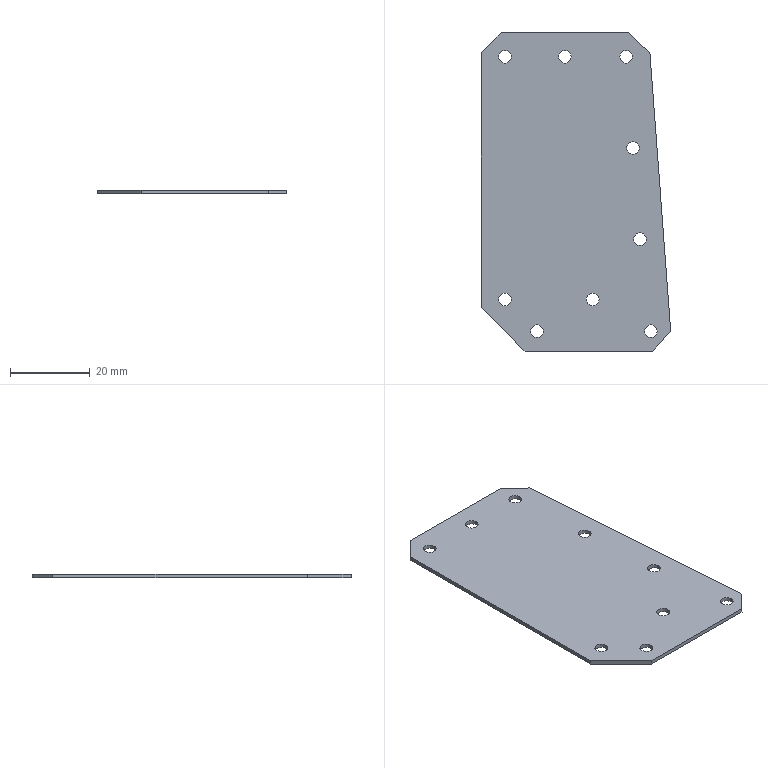Part | SolidWorks | features BaseBody 1 | 1 solid | 28 faces | box 47.626 x 80 x 1 mm | volume 3430 mm3 | cylinder 18 | plane 10 | commonest cylinder face diameters 3.2 x18
STEP:
#1=CARTESIAN_POINT('',(41.473,28.129,-1.));
#2=VERTEX_POINT('',#1);
#3=CARTESIAN_POINT('',(38.273,28.129,-1.));
#4=VERTEX_POINT('',#3);
#5=CARTESIAN_POINT('',(39.873,28.129,-1.));
#6=DIRECTION('',(0.,0.,-1.));
#7=DIRECTION('',(1.,0.,0.));
#8=AXIS2_PLACEMENT_3D('',#5,#6,#7);
#9=CIRCLE('',#8,1.6);
#10=EDGE_CURVE('',#2,#4,#9,.T.);
#11=ORIENTED_EDGE('',*,*,#10,.T.);
#12=CARTESIAN_POINT('',(38.273,28.129,0.));
#13=VERTEX_POINT('',#12);
#14=CARTESIAN_POINT('',(38.273,28.129,-1.));
#15=DIRECTION('',(0.,0.,1.));
#16=VECTOR('',#15,1000.);
#17=LINE('',#14,#16);
#18=EDGE_CURVE('',#4,#13,#17,.T.);
#19=ORIENTED_EDGE('',*,*,#18,.T.);
#20=CARTESIAN_POINT('',(41.473,28.129,0.));
#21=VERTEX_POINT('',#20);
#22=CARTESIAN_POINT('',(39.873,28.129,0.));
#23=DIRECTION('',(0.,0.,1.));
#24=DIRECTION('',(1.,0.,0.));
#25=AXIS2_PLACEMENT_3D('',#22,#23,#24);
#26=CIRCLE('',#25,1.6);
#27=EDGE_CURVE('',#13,#21,#26,.T.);
#28=ORIENTED_EDGE('',*,*,#27,.T.);
#29=CARTESIAN_POINT('',(41.473,28.129,-1.));
#30=DIRECTION('',(0.,0.,1.));
#31=VECTOR('',#30,1000.);
#32=LINE('',#29,#31);
#33=EDGE_CURVE('',#2,#21,#32,.T.);
#34=ORIENTED_EDGE('',*,*,#33,.F.);
#35=EDGE_LOOP('',(#11,#19,#28,#34));
#36=FACE_OUTER_BOUND('',#35,.T.);
#37=CARTESIAN_POINT('',(39.873,28.129,-1.));
#38=DIRECTION('',(0.,0.,1.));
#39=DIRECTION('',(1.,0.,0.));
#40=AXIS2_PLACEMENT_3D('',#37,#38,#39);
#41=CYLINDRICAL_SURFACE('',#40,1.6);
#42=ADVANCED_FACE('',(#36),#41,.F.);
#43=CARTESIAN_POINT('',(44.211,5.,-1.));
#44=VERTEX_POINT('',#43);
#45=CARTESIAN_POINT('',(41.011,5.,-1.));
#46=VERTEX_POINT('',#45);
#47=CARTESIAN_POINT('',(42.611,5.,-1.));
#48=DIRECTION('',(0.,0.,-1.));
#49=DIRECTION('',(1.,0.,0.));
#50=AXIS2_PLACEMENT_3D('',#47,#48,#49);
#51=CIRCLE('',#50,1.6);
#52=EDGE_CURVE('',#44,#46,#51,.T.);
#53=ORIENTED_EDGE('',*,*,#52,.T.);
#54=CARTESIAN_POINT('',(41.011,5.,0.));
#55=VERTEX_POINT('',#54);
#56=CARTESIAN_POINT('',(41.011,5.,-1.));
#57=DIRECTION('',(0.,0.,1.));
#58=VECTOR('',#57,1000.);
#59=LINE('',#56,#58);
#60=EDGE_CURVE('',#46,#55,#59,.T.);
#61=ORIENTED_EDGE('',*,*,#60,.T.);
#62=CARTESIAN_POINT('',(44.211,5.,0.));
#63=VERTEX_POINT('',#62);
#64=CARTESIAN_POINT('',(42.611,5.,0.));
#65=DIRECTION('',(0.,0.,-1.));
#66=DIRECTION('',(1.,0.,0.));
#67=AXIS2_PLACEMENT_3D('',#64,#65,#66);
#68=CIRCLE('',#67,1.6);
#69=EDGE_CURVE('',#63,#55,#68,.T.);
#70=ORIENTED_EDGE('',*,*,#69,.F.);
#71=CARTESIAN_POINT('',(44.211,5.,-1.));
#72=DIRECTION('',(0.,0.,1.));
#73=VECTOR('',#72,1000.);
#74=LINE('',#71,#73);
#75=EDGE_CURVE('',#44,#63,#74,.T.);
#76=ORIENTED_EDGE('',*,*,#75,.F.);
#77=EDGE_LOOP('',(#53,#61,#70,#76));
#78=FACE_OUTER_BOUND('',#77,.T.);
#79=CARTESIAN_POINT('',(42.611,5.,-1.));
#80=DIRECTION('',(0.,0.,1.));
#81=DIRECTION('',(1.,0.,0.));
#82=AXIS2_PLACEMENT_3D('',#79,#80,#81);
#83=CYLINDRICAL_SURFACE('',#82,1.6);
#84=ADVANCED_FACE('',(#78),#83,.F.);
#85=CARTESIAN_POINT('',(15.6,5.,-1.));
#86=VERTEX_POINT('',#85);
#87=CARTESIAN_POINT('',(12.4,5.,-1.));
#88=VERTEX_POINT('',#87);
#89=CARTESIAN_POINT('',(14.,5.,-1.));
#90=DIRECTION('',(0.,0.,-1.));
#91=DIRECTION('',(1.,0.,0.));
#92=AXIS2_PLACEMENT_3D('',#89,#90,#91);
#93=CIRCLE('',#92,1.6);
#94=EDGE_CURVE('',#86,#88,#93,.T.);
#95=ORIENTED_EDGE('',*,*,#94,.T.);
#96=CARTESIAN_POINT('',(12.4,5.,0.));
#97=VERTEX_POINT('',#96);
#98=CARTESIAN_POINT('',(12.4,5.,-1.));
#99=DIRECTION('',(0.,0.,1.));
#100=VECTOR('',#99,1000.);
#101=LINE('',#98,#100);
#102=EDGE_CURVE('',#88,#97,#101,.T.);
#103=ORIENTED_EDGE('',*,*,#102,.T.);
#104=CARTESIAN_POINT('',(15.6,5.,0.));
#105=VERTEX_POINT('',#104);
#106=CARTESIAN_POINT('',(14.,5.,0.));
#107=DIRECTION('',(0.,0.,-1.));
#108=DIRECTION('',(1.,0.,0.));
#109=AXIS2_PLACEMENT_3D('',#106,#107,#108);
#110=CIRCLE('',#109,1.6);
#111=EDGE_CURVE('',#105,#97,#110,.T.);
#112=ORIENTED_EDGE('',*,*,#111,.F.);
#113=CARTESIAN_POINT('',(15.6,5.,-1.));
#114=DIRECTION('',(0.,0.,1.));
#115=VECTOR('',#114,1000.);
#116=LINE('',#113,#115);
#117=EDGE_CURVE('',#86,#105,#116,.T.);
#118=ORIENTED_EDGE('',*,*,#117,.F.);
#119=EDGE_LOOP('',(#95,#103,#112,#118));
#120=FACE_OUTER_BOUND('',#119,.T.);
#121=CARTESIAN_POINT('',(14.,5.,-1.));
#122=DIRECTION('',(0.,0.,1.));
#123=DIRECTION('',(1.,0.,0.));
#124=AXIS2_PLACEMENT_3D('',#121,#122,#123);
#125=CYLINDRICAL_SURFACE('',#124,1.6);
#126=ADVANCED_FACE('',(#120),#125,.F.);
#127=CARTESIAN_POINT('',(7.6,13.,-1.));
#128=VERTEX_POINT('',#127);
#129=CARTESIAN_POINT('',(4.4,13.,-1.));
#130=VERTEX_POINT('',#129);
#131=CARTESIAN_POINT('',(6.,13.,-1.));
#132=DIRECTION('',(0.,0.,-1.));
#133=DIRECTION('',(1.,0.,0.));
#134=AXIS2_PLACEMENT_3D('',#131,#132,#133);
#135=CIRCLE('',#134,1.6);
#136=EDGE_CURVE('',#128,#130,#135,.T.);
#137=ORIENTED_EDGE('',*,*,#136,.T.);
#138=CARTESIAN_POINT('',(4.4,13.,0.));
#139=VERTEX_POINT('',#138);
#140=CARTESIAN_POINT('',(4.4,13.,-1.));
#141=DIRECTION('',(0.,0.,1.));
#142=VECTOR('',#141,1000.);
#143=LINE('',#140,#142);
#144=EDGE_CURVE('',#130,#139,#143,.T.);
#145=ORIENTED_EDGE('',*,*,#144,.T.);
#146=CARTESIAN_POINT('',(7.6,13.,0.));
#147=VERTEX_POINT('',#146);
#148=CARTESIAN_POINT('',(6.,13.,0.));
#149=DIRECTION('',(0.,0.,-1.));
#150=DIRECTION('',(1.,0.,0.));
#151=AXIS2_PLACEMENT_3D('',#148,#149,#150);
#152=CIRCLE('',#151,1.6);
#153=EDGE_CURVE('',#147,#139,#152,.T.);
#154=ORIENTED_EDGE('',*,*,#153,.F.);
#155=CARTESIAN_POINT('',(7.6,13.,-1.));
#156=DIRECTION('',(0.,0.,1.));
#157=VECTOR('',#156,1000.);
#158=LINE('',#155,#157);
#159=EDGE_CURVE('',#128,#147,#158,.T.);
#160=ORIENTED_EDGE('',*,*,#159,.F.);
#161=EDGE_LOOP('',(#137,#145,#154,#160));
#162=FACE_OUTER_BOUND('',#161,.T.);
#163=CARTESIAN_POINT('',(6.,13.,-1.));
#164=DIRECTION('',(0.,0.,1.));
#165=DIRECTION('',(1.,0.,0.));
#166=AXIS2_PLACEMENT_3D('',#163,#164,#165);
#167=CYLINDRICAL_SURFACE('',#166,1.6);
#168=ADVANCED_FACE('',(#162),#167,.F.);
#169=CARTESIAN_POINT('',(29.6,13.,-1.));
#170=VERTEX_POINT('',#169);
#171=CARTESIAN_POINT('',(26.4,13.,-1.));
#172=VERTEX_POINT('',#171);
#173=CARTESIAN_POINT('',(28.,13.,-1.));
#174=DIRECTION('',(0.,0.,-1.));
#175=DIRECTION('',(1.,0.,0.));
#176=AXIS2_PLACEMENT_3D('',#173,#174,#175);
#177=CIRCLE('',#176,1.6);
#178=EDGE_CURVE('',#170,#172,#177,.T.);
#179=ORIENTED_EDGE('',*,*,#178,.T.);
#180=CARTESIAN_POINT('',(26.4,13.,0.));
#181=VERTEX_POINT('',#180);
#182=CARTESIAN_POINT('',(26.4,13.,-1.));
#183=DIRECTION('',(0.,0.,1.));
#184=VECTOR('',#183,1000.);
#185=LINE('',#182,#184);
#186=EDGE_CURVE('',#172,#181,#185,.T.);
#187=ORIENTED_EDGE('',*,*,#186,.T.);
#188=CARTESIAN_POINT('',(29.6,13.,0.));
#189=VERTEX_POINT('',#188);
#190=CARTESIAN_POINT('',(28.,13.,0.));
#191=DIRECTION('',(0.,0.,-1.));
#192=DIRECTION('',(1.,0.,0.));
#193=AXIS2_PLACEMENT_3D('',#190,#191,#192);
#194=CIRCLE('',#193,1.6);
#195=EDGE_CURVE('',#189,#181,#194,.T.);
#196=ORIENTED_EDGE('',*,*,#195,.F.);
#197=CARTESIAN_POINT('',(29.6,13.,-1.));
#198=DIRECTION('',(0.,0.,1.));
#199=VECTOR('',#198,1000.);
#200=LINE('',#197,#199);
#201=EDGE_CURVE('',#170,#189,#200,.T.);
#202=ORIENTED_EDGE('',*,*,#201,.F.);
#203=EDGE_LOOP('',(#179,#187,#196,#202));
#204=FACE_OUTER_BOUND('',#203,.T.);
#205=CARTESIAN_POINT('',(28.,13.,-1.));
#206=DIRECTION('',(0.,0.,1.));
#207=DIRECTION('',(1.,0.,0.));
#208=AXIS2_PLACEMENT_3D('',#205,#206,#207);
#209=CYLINDRICAL_SURFACE('',#208,1.6);
#210=ADVANCED_FACE('',(#204),#209,.F.);
#211=CARTESIAN_POINT('',(7.6,74.,-1.));
#212=VERTEX_POINT('',#211);
#213=CARTESIAN_POINT('',(4.4,74.,-1.));
#214=VERTEX_POINT('',#213);
#215=CARTESIAN_POINT('',(6.,74.,-1.));
#216=DIRECTION('',(0.,0.,-1.));
#217=DIRECTION('',(1.,0.,0.));
#218=AXIS2_PLACEMENT_3D('',#215,#216,#217);
#219=CIRCLE('',#218,1.6);
#220=EDGE_CURVE('',#212,#214,#219,.T.);
#221=ORIENTED_EDGE('',*,*,#220,.T.);
#222=CARTESIAN_POINT('',(4.4,74.,0.));
#223=VERTEX_POINT('',#222);
#224=CARTESIAN_POINT('',(4.4,74.,-1.));
#225=DIRECTION('',(0.,0.,1.));
#226=VECTOR('',#225,1000.);
#227=LINE('',#224,#226);
#228=EDGE_CURVE('',#214,#223,#227,.T.);
#229=ORIENTED_EDGE('',*,*,#228,.T.);
#230=CARTESIAN_POINT('',(7.6,74.,0.));
#231=VERTEX_POINT('',#230);
#232=CARTESIAN_POINT('',(6.,74.,0.));
#233=DIRECTION('',(0.,0.,-1.));
#234=DIRECTION('',(1.,0.,0.));
#235=AXIS2_PLACEMENT_3D('',#232,#233,#234);
#236=CIRCLE('',#235,1.6);
#237=EDGE_CURVE('',#231,#223,#236,.T.);
#238=ORIENTED_EDGE('',*,*,#237,.F.);
#239=CARTESIAN_POINT('',(7.6,74.,-1.));
#240=DIRECTION('',(0.,0.,1.));
#241=VECTOR('',#240,1000.);
#242=LINE('',#239,#241);
#243=EDGE_CURVE('',#212,#231,#242,.T.);
#244=ORIENTED_EDGE('',*,*,#243,.F.);
#245=EDGE_LOOP('',(#221,#229,#238,#244));
#246=FACE_OUTER_BOUND('',#245,.T.);
#247=CARTESIAN_POINT('',(6.,74.,-1.));
#248=DIRECTION('',(0.,0.,1.));
#249=DIRECTION('',(1.,0.,0.));
#250=AXIS2_PLACEMENT_3D('',#247,#248,#249);
#251=CYLINDRICAL_SURFACE('',#250,1.6);
#252=ADVANCED_FACE('',(#246),#251,.F.);
#253=CARTESIAN_POINT('',(22.6,74.,-1.));
#254=VERTEX_POINT('',#253);
#255=CARTESIAN_POINT('',(19.4,74.,-1.));
#256=VERTEX_POINT('',#255);
#257=CARTESIAN_POINT('',(21.,74.,-1.));
#258=DIRECTION('',(0.,0.,-1.));
#259=DIRECTION('',(1.,0.,0.));
#260=AXIS2_PLACEMENT_3D('',#257,#258,#259);
#261=CIRCLE('',#260,1.6);
#262=EDGE_CURVE('',#254,#256,#261,.T.);
#263=ORIENTED_EDGE('',*,*,#262,.T.);
#264=CARTESIAN_POINT('',(19.4,74.,0.));
#265=VERTEX_POINT('',#264);
#266=CARTESIAN_POINT('',(19.4,74.,-1.));
#267=DIRECTION('',(0.,0.,1.));
#268=VECTOR('',#267,1000.);
#269=LINE('',#266,#268);
#270=EDGE_CURVE('',#256,#265,#269,.T.);
#271=ORIENTED_EDGE('',*,*,#270,.T.);
#272=CARTESIAN_POINT('',(22.6,74.,0.));
#273=VERTEX_POINT('',#272);
#274=CARTESIAN_POINT('',(21.,74.,0.));
#275=DIRECTION('',(0.,0.,-1.));
#276=DIRECTION('',(1.,0.,0.));
#277=AXIS2_PLACEMENT_3D('',#274,#275,#276);
#278=CIRCLE('',#277,1.6);
#279=EDGE_CURVE('',#273,#265,#278,.T.);
#280=ORIENTED_EDGE('',*,*,#279,.F.);
#281=CARTESIAN_POINT('',(22.6,74.,-1.));
#282=DIRECTION('',(0.,0.,1.));
#283=VECTOR('',#282,1000.);
#284=LINE('',#281,#283);
#285=EDGE_CURVE('',#254,#273,#284,.T.);
#286=ORIENTED_EDGE('',*,*,#285,.F.);
#287=EDGE_LOOP('',(#263,#271,#280,#286));
#288=FACE_OUTER_BOUND('',#287,.T.);
#289=CARTESIAN_POINT('',(21.,74.,-1.));
#290=DIRECTION('',(0.,0.,1.));
#291=DIRECTION('',(1.,0.,0.));
#292=AXIS2_PLACEMENT_3D('',#289,#290,#291);
#293=CYLINDRICAL_SURFACE('',#292,1.6);
#294=ADVANCED_FACE('',(#288),#293,.F.);
#295=CARTESIAN_POINT('',(38.033,74.,-1.));
#296=VERTEX_POINT('',#295);
#297=CARTESIAN_POINT('',(34.833,74.,-1.));
#298=VERTEX_POINT('',#297);
#299=CARTESIAN_POINT('',(36.433,74.,-1.));
#300=DIRECTION('',(0.,0.,-1.));
#301=DIRECTION('',(1.,0.,0.));
#302=AXIS2_PLACEMENT_3D('',#299,#300,#301);
#303=CIRCLE('',#302,1.6);
#304=EDGE_CURVE('',#296,#298,#303,.T.);
#305=ORIENTED_EDGE('',*,*,#304,.T.);
#306=CARTESIAN_POINT('',(34.833,74.,0.));
#307=VERTEX_POINT('',#306);
#308=CARTESIAN_POINT('',(34.833,74.,-1.));
#309=DIRECTION('',(0.,0.,1.));
#310=VECTOR('',#309,1000.);
#311=LINE('',#308,#310);
#312=EDGE_CURVE('',#298,#307,#311,.T.);
#313=ORIENTED_EDGE('',*,*,#312,.T.);
#314=CARTESIAN_POINT('',(38.033,74.,0.));
#315=VERTEX_POINT('',#314);
#316=CARTESIAN_POINT('',(36.433,74.,0.));
#317=DIRECTION('',(0.,0.,-1.));
#318=DIRECTION('',(1.,0.,0.));
#319=AXIS2_PLACEMENT_3D('',#316,#317,#318);
#320=CIRCLE('',#319,1.6);
#321=EDGE_CURVE('',#315,#307,#320,.T.);
#322=ORIENTED_EDGE('',*,*,#321,.F.);
#323=CARTESIAN_POINT('',(38.033,74.,-1.));
#324=DIRECTION('',(0.,0.,1.));
#325=VECTOR('',#324,1000.);
#326=LINE('',#323,#325);
#327=EDGE_CURVE('',#296,#315,#326,.T.);
#328=ORIENTED_EDGE('',*,*,#327,.F.);
#329=EDGE_LOOP('',(#305,#313,#322,#328));
#330=FACE_OUTER_BOUND('',#329,.T.);
#331=CARTESIAN_POINT('',(36.433,74.,-1.));
#332=DIRECTION('',(0.,0.,1.));
#333=DIRECTION('',(1.,0.,0.));
#334=AXIS2_PLACEMENT_3D('',#331,#332,#333);
#335=CYLINDRICAL_SURFACE('',#334,1.6);
#336=ADVANCED_FACE('',(#330),#335,.F.);
#337=CARTESIAN_POINT('',(39.753,51.064,-1.));
#338=VERTEX_POINT('',#337);
#339=CARTESIAN_POINT('',(36.553,51.064,-1.));
#340=VERTEX_POINT('',#339);
#341=CARTESIAN_POINT('',(38.153,51.064,-1.));
#342=DIRECTION('',(0.,0.,-1.));
#343=DIRECTION('',(1.,0.,0.));
#344=AXIS2_PLACEMENT_3D('',#341,#342,#343);
#345=CIRCLE('',#344,1.6);
#346=EDGE_CURVE('',#338,#340,#345,.T.);
#347=ORIENTED_EDGE('',*,*,#346,.T.);
#348=CARTESIAN_POINT('',(36.553,51.064,0.));
#349=VERTEX_POINT('',#348);
#350=CARTESIAN_POINT('',(36.553,51.064,-1.));
#351=DIRECTION('',(0.,0.,1.));
#352=VECTOR('',#351,1000.);
#353=LINE('',#350,#352);
#354=EDGE_CURVE('',#340,#349,#353,.T.);
#355=ORIENTED_EDGE('',*,*,#354,.T.);
#356=CARTESIAN_POINT('',(39.753,51.064,0.));
#357=VERTEX_POINT('',#356);
#358=CARTESIAN_POINT('',(38.153,51.064,0.));
#359=DIRECTION('',(0.,0.,-1.));
#360=DIRECTION('',(1.,0.,0.));
#361=AXIS2_PLACEMENT_3D('',#358,#359,#360);
#362=CIRCLE('',#361,1.6);
#363=EDGE_CURVE('',#357,#349,#362,.T.);
#364=ORIENTED_EDGE('',*,*,#363,.F.);
#365=CARTESIAN_POINT('',(39.753,51.064,-1.));
#366=DIRECTION('',(0.,0.,1.));
#367=VECTOR('',#366,1000.);
#368=LINE('',#365,#367);
#369=EDGE_CURVE('',#338,#357,#368,.T.);
#370=ORIENTED_EDGE('',*,*,#369,.F.);
#371=EDGE_LOOP('',(#347,#355,#364,#370));
#372=FACE_OUTER_BOUND('',#371,.T.);
#373=CARTESIAN_POINT('',(38.153,51.064,-1.));
#374=DIRECTION('',(0.,0.,1.));
#375=DIRECTION('',(1.,0.,0.));
#376=AXIS2_PLACEMENT_3D('',#373,#374,#375);
#377=CYLINDRICAL_SURFACE('',#376,1.6);
#378=ADVANCED_FACE('',(#372),#377,.F.);
#379=ORIENTED_EDGE('',*,*,#18,.F.);
#380=CARTESIAN_POINT('',(39.873,28.129,-1.));
#381=DIRECTION('',(0.,0.,-1.));
#382=DIRECTION('',(1.,0.,0.));
#383=AXIS2_PLACEMENT_3D('',#380,#381,#382);
#384=CIRCLE('',#383,1.6);
#385=EDGE_CURVE('',#4,#2,#384,.T.);
#386=ORIENTED_EDGE('',*,*,#385,.T.);
#387=ORIENTED_EDGE('',*,*,#33,.T.);
#388=CARTESIAN_POINT('',(39.873,28.129,0.));
#389=DIRECTION('',(0.,0.,1.));
#390=DIRECTION('',(1.,0.,0.));
#391=AXIS2_PLACEMENT_3D('',#388,#389,#390);
#392=CIRCLE('',#391,1.6);
#393=EDGE_CURVE('',#21,#13,#392,.T.);
#394=ORIENTED_EDGE('',*,*,#393,.T.);
#395=EDGE_LOOP('',(#379,#386,#387,#394));
#396=FACE_OUTER_BOUND('',#395,.T.);
#397=CARTESIAN_POINT('',(39.873,28.129,-1.));
#398=DIRECTION('',(0.,0.,1.));
#399=DIRECTION('',(1.,0.,0.));
#400=AXIS2_PLACEMENT_3D('',#397,#398,#399);
#401=CYLINDRICAL_SURFACE('',#400,1.6);
#402=ADVANCED_FACE('',(#396),#401,.F.);
#403=ORIENTED_EDGE('',*,*,#69,.T.);
#404=CARTESIAN_POINT('',(42.611,5.,0.));
#405=DIRECTION('',(0.,0.,-1.));
#406=DIRECTION('',(1.,0.,0.));
#407=AXIS2_PLACEMENT_3D('',#404,#405,#406);
#408=CIRCLE('',#407,1.6);
#409=EDGE_CURVE('',#55,#63,#408,.T.);
#410=ORIENTED_EDGE('',*,*,#409,.T.);
#411=EDGE_LOOP('',(#403,#410));
#412=FACE_BOUND('',#411,.T.);
#413=ORIENTED_EDGE('',*,*,#111,.T.);
#414=CARTESIAN_POINT('',(14.,5.,0.));
#415=DIRECTION('',(0.,0.,-1.));
#416=DIRECTION('',(1.,0.,0.));
#417=AXIS2_PLACEMENT_3D('',#414,#415,#416);
#418=CIRCLE('',#417,1.6);
#419=EDGE_CURVE('',#97,#105,#418,.T.);
#420=ORIENTED_EDGE('',*,*,#419,.T.);
#421=EDGE_LOOP('',(#413,#420));
#422=FACE_BOUND('',#421,.T.);
#423=ORIENTED_EDGE('',*,*,#153,.T.);
#424=CARTESIAN_POINT('',(6.,13.,0.));
#425=DIRECTION('',(0.,0.,-1.));
#426=DIRECTION('',(1.,0.,0.));
#427=AXIS2_PLACEMENT_3D('',#424,#425,#426);
#428=CIRCLE('',#427,1.6);
#429=EDGE_CURVE('',#139,#147,#428,.T.);
#430=ORIENTED_EDGE('',*,*,#429,.T.);
#431=EDGE_LOOP('',(#423,#430));
#432=FACE_BOUND('',#431,.T.);
#433=ORIENTED_EDGE('',*,*,#195,.T.);
#434=CARTESIAN_POINT('',(28.,13.,0.));
#435=DIRECTION('',(0.,0.,-1.));
#436=DIRECTION('',(1.,0.,0.));
#437=AXIS2_PLACEMENT_3D('',#434,#435,#436);
#438=CIRCLE('',#437,1.6);
#439=EDGE_CURVE('',#181,#189,#438,.T.);
#440=ORIENTED_EDGE('',*,*,#439,.T.);
#441=EDGE_LOOP('',(#433,#440));
#442=FACE_BOUND('',#441,.T.);
#443=ORIENTED_EDGE('',*,*,#237,.T.);
#444=CARTESIAN_POINT('',(6.,74.,0.));
#445=DIRECTION('',(0.,0.,-1.));
#446=DIRECTION('',(1.,0.,0.));
#447=AXIS2_PLACEMENT_3D('',#444,#445,#446);
#448=CIRCLE('',#447,1.6);
#449=EDGE_CURVE('',#223,#231,#448,.T.);
#450=ORIENTED_EDGE('',*,*,#449,.T.);
#451=EDGE_LOOP('',(#443,#450));
#452=FACE_BOUND('',#451,.T.);
#453=ORIENTED_EDGE('',*,*,#279,.T.);
#454=CARTESIAN_POINT('',(21.,74.,0.));
#455=DIRECTION('',(0.,0.,-1.));
#456=DIRECTION('',(1.,0.,0.));
#457=AXIS2_PLACEMENT_3D('',#454,#455,#456);
#458=CIRCLE('',#457,1.6);
#459=EDGE_CURVE('',#265,#273,#458,.T.);
#460=ORIENTED_EDGE('',*,*,#459,.T.);
#461=EDGE_LOOP('',(#453,#460));
#462=FACE_BOUND('',#461,.T.);
#463=ORIENTED_EDGE('',*,*,#321,.T.);
#464=CARTESIAN_POINT('',(36.433,74.,0.));
#465=DIRECTION('',(0.,0.,-1.));
#466=DIRECTION('',(1.,0.,0.));
#467=AXIS2_PLACEMENT_3D('',#464,#465,#466);
#468=CIRCLE('',#467,1.6);
#469=EDGE_CURVE('',#307,#315,#468,.T.);
#470=ORIENTED_EDGE('',*,*,#469,.T.);
#471=EDGE_LOOP('',(#463,#470));
#472=FACE_BOUND('',#471,.T.);
#473=ORIENTED_EDGE('',*,*,#363,.T.);
#474=CARTESIAN_POINT('',(38.153,51.064,0.));
#475=DIRECTION('',(0.,0.,-1.));
#476=DIRECTION('',(1.,0.,0.));
#477=AXIS2_PLACEMENT_3D('',#474,#475,#476);
#478=CIRCLE('',#477,1.6);
#479=EDGE_CURVE('',#349,#357,#478,.T.);
#480=ORIENTED_EDGE('',*,*,#479,.T.);
#481=EDGE_LOOP('',(#473,#480));
#482=FACE_BOUND('',#481,.T.);
#483=ORIENTED_EDGE('',*,*,#393,.F.);
#484=ORIENTED_EDGE('',*,*,#27,.F.);
#485=EDGE_LOOP('',(#483,#484));
#486=FACE_BOUND('',#485,.T.);
#487=CARTESIAN_POINT('',(0.,75.,0.));
#488=VERTEX_POINT('',#487);
#489=CARTESIAN_POINT('',(0.,11.,0.));
#490=VERTEX_POINT('',#489);
#491=CARTESIAN_POINT('',(0.,40.,0.));
#492=DIRECTION('',(0.,-1.,0.));
#493=VECTOR('',#492,1000.);
#494=LINE('',#491,#493);
#495=EDGE_CURVE('',#488,#490,#494,.T.);
#496=ORIENTED_EDGE('',*,*,#495,.T.);
#497=CARTESIAN_POINT('',(11.,0.,0.));
#498=VERTEX_POINT('',#497);
#499=CARTESIAN_POINT('',(0.,11.,0.));
#500=DIRECTION('',(0.7071,-0.7071,0.));
#501=VECTOR('',#500,1000.);
#502=LINE('',#499,#501);
#503=EDGE_CURVE('',#490,#498,#502,.T.);
#504=ORIENTED_EDGE('',*,*,#503,.T.);
#505=CARTESIAN_POINT('',(43.,0.,0.));
#506=VERTEX_POINT('',#505);
#507=CARTESIAN_POINT('',(23.956,0.,0.));
#508=DIRECTION('',(1.,0.,0.));
#509=VECTOR('',#508,1000.);
#510=LINE('',#507,#509);
#511=EDGE_CURVE('',#498,#506,#510,.T.);
#512=ORIENTED_EDGE('',*,*,#511,.T.);
#513=CARTESIAN_POINT('',(47.626,4.986,0.));
#514=VERTEX_POINT('',#513);
#515=CARTESIAN_POINT('',(43.,0.,0.));
#516=DIRECTION('',(0.6802,0.7331,0.));
#517=VECTOR('',#516,1000.);
#518=LINE('',#515,#517);
#519=EDGE_CURVE('',#506,#514,#518,.T.);
#520=ORIENTED_EDGE('',*,*,#519,.T.);
#521=CARTESIAN_POINT('',(42.374,75.014,0.));
#522=VERTEX_POINT('',#521);
#523=CARTESIAN_POINT('',(47.626,4.986,0.));
#524=DIRECTION('',(-0.07479,0.9972,0.));
#525=VECTOR('',#524,1000.);
#526=LINE('',#523,#525);
#527=EDGE_CURVE('',#514,#522,#526,.T.);
#528=ORIENTED_EDGE('',*,*,#527,.T.);
#529=CARTESIAN_POINT('',(37.,80.,0.));
#530=VERTEX_POINT('',#529);
#531=CARTESIAN_POINT('',(42.374,75.014,0.));
#532=DIRECTION('',(-0.7331,0.6802,0.));
#533=VECTOR('',#532,1000.);
#534=LINE('',#531,#533);
#535=EDGE_CURVE('',#522,#530,#534,.T.);
#536=ORIENTED_EDGE('',*,*,#535,.T.);
#537=CARTESIAN_POINT('',(5.,80.,0.));
#538=VERTEX_POINT('',#537);
#539=CARTESIAN_POINT('',(23.956,80.,0.));
#540=DIRECTION('',(-1.,0.,0.));
#541=VECTOR('',#540,1000.);
#542=LINE('',#539,#541);
#543=EDGE_CURVE('',#530,#538,#542,.T.);
#544=ORIENTED_EDGE('',*,*,#543,.T.);
#545=CARTESIAN_POINT('',(5.,80.,0.));
#546=DIRECTION('',(-0.7071,-0.7071,0.));
#547=VECTOR('',#546,1000.);
#548=LINE('',#545,#547);
#549=EDGE_CURVE('',#538,#488,#548,.T.);
#550=ORIENTED_EDGE('',*,*,#549,.T.);
#551=EDGE_LOOP('',(#496,#504,#512,#520,#528,#536,#544,#550));
#552=FACE_OUTER_BOUND('',#551,.T.);
#553=CARTESIAN_POINT('',(0.,0.,0.));
#554=DIRECTION('',(0.,0.,1.));
#555=DIRECTION('',(1.,0.,0.));
#556=AXIS2_PLACEMENT_3D('',#553,#554,#555);
#557=PLANE('',#556);
#558=ADVANCED_FACE('',(#412,#422,#432,#442,#452,#462,#472,#482,#486,#552),#557,.T.);
#559=ORIENTED_EDGE('',*,*,#52,.F.);
#560=CARTESIAN_POINT('',(42.611,5.,-1.));
#561=DIRECTION('',(0.,0.,-1.));
#562=DIRECTION('',(1.,0.,0.));
#563=AXIS2_PLACEMENT_3D('',#560,#561,#562);
#564=CIRCLE('',#563,1.6);
#565=EDGE_CURVE('',#46,#44,#564,.T.);
#566=ORIENTED_EDGE('',*,*,#565,.F.);
#567=EDGE_LOOP('',(#559,#566));
#568=FACE_BOUND('',#567,.T.);
#569=ORIENTED_EDGE('',*,*,#94,.F.);
#570=CARTESIAN_POINT('',(14.,5.,-1.));
#571=DIRECTION('',(0.,0.,-1.));
#572=DIRECTION('',(1.,0.,0.));
#573=AXIS2_PLACEMENT_3D('',#570,#571,#572);
#574=CIRCLE('',#573,1.6);
#575=EDGE_CURVE('',#88,#86,#574,.T.);
#576=ORIENTED_EDGE('',*,*,#575,.F.);
#577=EDGE_LOOP('',(#569,#576));
#578=FACE_BOUND('',#577,.T.);
#579=ORIENTED_EDGE('',*,*,#136,.F.);
#580=CARTESIAN_POINT('',(6.,13.,-1.));
#581=DIRECTION('',(0.,0.,-1.));
#582=DIRECTION('',(1.,0.,0.));
#583=AXIS2_PLACEMENT_3D('',#580,#581,#582);
#584=CIRCLE('',#583,1.6);
#585=EDGE_CURVE('',#130,#128,#584,.T.);
#586=ORIENTED_EDGE('',*,*,#585,.F.);
#587=EDGE_LOOP('',(#579,#586));
#588=FACE_BOUND('',#587,.T.);
#589=ORIENTED_EDGE('',*,*,#178,.F.);
#590=CARTESIAN_POINT('',(28.,13.,-1.));
#591=DIRECTION('',(0.,0.,-1.));
#592=DIRECTION('',(1.,0.,0.));
#593=AXIS2_PLACEMENT_3D('',#590,#591,#592);
#594=CIRCLE('',#593,1.6);
#595=EDGE_CURVE('',#172,#170,#594,.T.);
#596=ORIENTED_EDGE('',*,*,#595,.F.);
#597=EDGE_LOOP('',(#589,#596));
#598=FACE_BOUND('',#597,.T.);
#599=ORIENTED_EDGE('',*,*,#220,.F.);
#600=CARTESIAN_POINT('',(6.,74.,-1.));
#601=DIRECTION('',(0.,0.,-1.));
#602=DIRECTION('',(1.,0.,0.));
#603=AXIS2_PLACEMENT_3D('',#600,#601,#602);
#604=CIRCLE('',#603,1.6);
#605=EDGE_CURVE('',#214,#212,#604,.T.);
#606=ORIENTED_EDGE('',*,*,#605,.F.);
#607=EDGE_LOOP('',(#599,#606));
#608=FACE_BOUND('',#607,.T.);
#609=ORIENTED_EDGE('',*,*,#262,.F.);
#610=CARTESIAN_POINT('',(21.,74.,-1.));
#611=DIRECTION('',(0.,0.,-1.));
#612=DIRECTION('',(1.,0.,0.));
#613=AXIS2_PLACEMENT_3D('',#610,#611,#612);
#614=CIRCLE('',#613,1.6);
#615=EDGE_CURVE('',#256,#254,#614,.T.);
#616=ORIENTED_EDGE('',*,*,#615,.F.);
#617=EDGE_LOOP('',(#609,#616));
#618=FACE_BOUND('',#617,.T.);
#619=ORIENTED_EDGE('',*,*,#304,.F.);
#620=CARTESIAN_POINT('',(36.433,74.,-1.));
#621=DIRECTION('',(0.,0.,-1.));
#622=DIRECTION('',(1.,0.,0.));
#623=AXIS2_PLACEMENT_3D('',#620,#621,#622);
#624=CIRCLE('',#623,1.6);
#625=EDGE_CURVE('',#298,#296,#624,.T.);
#626=ORIENTED_EDGE('',*,*,#625,.F.);
#627=EDGE_LOOP('',(#619,#626));
#628=FACE_BOUND('',#627,.T.);
#629=ORIENTED_EDGE('',*,*,#346,.F.);
#630=CARTESIAN_POINT('',(38.153,51.064,-1.));
#631=DIRECTION('',(0.,0.,-1.));
#632=DIRECTION('',(1.,0.,0.));
#633=AXIS2_PLACEMENT_3D('',#630,#631,#632);
#634=CIRCLE('',#633,1.6);
#635=EDGE_CURVE('',#340,#338,#634,.T.);
#636=ORIENTED_EDGE('',*,*,#635,.F.);
#637=EDGE_LOOP('',(#629,#636));
#638=FACE_BOUND('',#637,.T.);
#639=ORIENTED_EDGE('',*,*,#10,.F.);
#640=ORIENTED_EDGE('',*,*,#385,.F.);
#641=EDGE_LOOP('',(#639,#640));
#642=FACE_BOUND('',#641,.T.);
#643=CARTESIAN_POINT('',(43.,0.,-1.));
#644=VERTEX_POINT('',#643);
#645=CARTESIAN_POINT('',(47.626,4.986,-1.));
#646=VERTEX_POINT('',#645);
#647=CARTESIAN_POINT('',(47.626,4.986,-1.));
#648=DIRECTION('',(0.6802,0.7331,0.));
#649=VECTOR('',#648,1000.);
#650=LINE('',#647,#649);
#651=EDGE_CURVE('',#644,#646,#650,.T.);
#652=ORIENTED_EDGE('',*,*,#651,.F.);
#653=CARTESIAN_POINT('',(11.,0.,-1.));
#654=VERTEX_POINT('',#653);
#655=CARTESIAN_POINT('',(23.956,0.,-1.));
#656=DIRECTION('',(1.,0.,0.));
#657=VECTOR('',#656,1000.);
#658=LINE('',#655,#657);
#659=EDGE_CURVE('',#654,#644,#658,.T.);
#660=ORIENTED_EDGE('',*,*,#659,.F.);
#661=CARTESIAN_POINT('',(0.,11.,-1.));
#662=VERTEX_POINT('',#661);
#663=CARTESIAN_POINT('',(0.,11.,-1.));
#664=DIRECTION('',(0.7071,-0.7071,0.));
#665=VECTOR('',#664,1000.);
#666=LINE('',#663,#665);
#667=EDGE_CURVE('',#662,#654,#666,.T.);
#668=ORIENTED_EDGE('',*,*,#667,.F.);
#669=CARTESIAN_POINT('',(0.,75.,-1.));
#670=VERTEX_POINT('',#669);
#671=CARTESIAN_POINT('',(0.,40.,-1.));
#672=DIRECTION('',(0.,-1.,0.));
#673=VECTOR('',#672,1000.);
#674=LINE('',#671,#673);
#675=EDGE_CURVE('',#670,#662,#674,.T.);
#676=ORIENTED_EDGE('',*,*,#675,.F.);
#677=CARTESIAN_POINT('',(5.,80.,-1.));
#678=VERTEX_POINT('',#677);
#679=CARTESIAN_POINT('',(0.,75.,-1.));
#680=DIRECTION('',(-0.7071,-0.7071,0.));
#681=VECTOR('',#680,1000.);
#682=LINE('',#679,#681);
#683=EDGE_CURVE('',#678,#670,#682,.T.);
#684=ORIENTED_EDGE('',*,*,#683,.F.);
#685=CARTESIAN_POINT('',(37.,80.,-1.));
#686=VERTEX_POINT('',#685);
#687=CARTESIAN_POINT('',(23.956,80.,-1.));
#688=DIRECTION('',(-1.,0.,0.));
#689=VECTOR('',#688,1000.);
#690=LINE('',#687,#689);
#691=EDGE_CURVE('',#686,#678,#690,.T.);
#692=ORIENTED_EDGE('',*,*,#691,.F.);
#693=CARTESIAN_POINT('',(42.374,75.014,-1.));
#694=VERTEX_POINT('',#693);
#695=CARTESIAN_POINT('',(37.,80.,-1.));
#696=DIRECTION('',(-0.7331,0.6802,0.));
#697=VECTOR('',#696,1000.);
#698=LINE('',#695,#697);
#699=EDGE_CURVE('',#694,#686,#698,.T.);
#700=ORIENTED_EDGE('',*,*,#699,.F.);
#701=CARTESIAN_POINT('',(47.626,4.986,-1.));
#702=DIRECTION('',(-0.07479,0.9972,0.));
#703=VECTOR('',#702,1000.);
#704=LINE('',#701,#703);
#705=EDGE_CURVE('',#646,#694,#704,.T.);
#706=ORIENTED_EDGE('',*,*,#705,.F.);
#707=EDGE_LOOP('',(#652,#660,#668,#676,#684,#692,#700,#706));
#708=FACE_OUTER_BOUND('',#707,.T.);
#709=CARTESIAN_POINT('',(0.,0.,-1.));
#710=DIRECTION('',(0.,0.,1.));
#711=DIRECTION('',(1.,0.,0.));
#712=AXIS2_PLACEMENT_3D('',#709,#710,#711);
#713=PLANE('',#712);
#714=ADVANCED_FACE('',(#568,#578,#588,#598,#608,#618,#628,#638,#642,#708),#713,.F.);
#715=ORIENTED_EDGE('',*,*,#60,.F.);
#716=ORIENTED_EDGE('',*,*,#565,.T.);
#717=ORIENTED_EDGE('',*,*,#75,.T.);
#718=ORIENTED_EDGE('',*,*,#409,.F.);
#719=EDGE_LOOP('',(#715,#716,#717,#718));
#720=FACE_OUTER_BOUND('',#719,.T.);
#721=CARTESIAN_POINT('',(42.611,5.,-1.));
#722=DIRECTION('',(0.,0.,1.));
#723=DIRECTION('',(1.,0.,0.));
#724=AXIS2_PLACEMENT_3D('',#721,#722,#723);
#725=CYLINDRICAL_SURFACE('',#724,1.6);
#726=ADVANCED_FACE('',(#720),#725,.F.);
#727=ORIENTED_EDGE('',*,*,#102,.F.);
#728=ORIENTED_EDGE('',*,*,#575,.T.);
#729=ORIENTED_EDGE('',*,*,#117,.T.);
#730=ORIENTED_EDGE('',*,*,#419,.F.);
#731=EDGE_LOOP('',(#727,#728,#729,#730));
#732=FACE_OUTER_BOUND('',#731,.T.);
#733=CARTESIAN_POINT('',(14.,5.,-1.));
#734=DIRECTION('',(0.,0.,1.));
#735=DIRECTION('',(1.,0.,0.));
#736=AXIS2_PLACEMENT_3D('',#733,#734,#735);
#737=CYLINDRICAL_SURFACE('',#736,1.6);
#738=ADVANCED_FACE('',(#732),#737,.F.);
#739=ORIENTED_EDGE('',*,*,#144,.F.);
#740=ORIENTED_EDGE('',*,*,#585,.T.);
#741=ORIENTED_EDGE('',*,*,#159,.T.);
#742=ORIENTED_EDGE('',*,*,#429,.F.);
#743=EDGE_LOOP('',(#739,#740,#741,#742));
#744=FACE_OUTER_BOUND('',#743,.T.);
#745=CARTESIAN_POINT('',(6.,13.,-1.));
#746=DIRECTION('',(0.,0.,1.));
#747=DIRECTION('',(1.,0.,0.));
#748=AXIS2_PLACEMENT_3D('',#745,#746,#747);
#749=CYLINDRICAL_SURFACE('',#748,1.6);
#750=ADVANCED_FACE('',(#744),#749,.F.);
#751=ORIENTED_EDGE('',*,*,#186,.F.);
#752=ORIENTED_EDGE('',*,*,#595,.T.);
#753=ORIENTED_EDGE('',*,*,#201,.T.);
#754=ORIENTED_EDGE('',*,*,#439,.F.);
#755=EDGE_LOOP('',(#751,#752,#753,#754));
#756=FACE_OUTER_BOUND('',#755,.T.);
#757=CARTESIAN_POINT('',(28.,13.,-1.));
#758=DIRECTION('',(0.,0.,1.));
#759=DIRECTION('',(1.,0.,0.));
#760=AXIS2_PLACEMENT_3D('',#757,#758,#759);
#761=CYLINDRICAL_SURFACE('',#760,1.6);
#762=ADVANCED_FACE('',(#756),#761,.F.);
#763=ORIENTED_EDGE('',*,*,#228,.F.);
#764=ORIENTED_EDGE('',*,*,#605,.T.);
#765=ORIENTED_EDGE('',*,*,#243,.T.);
#766=ORIENTED_EDGE('',*,*,#449,.F.);
#767=EDGE_LOOP('',(#763,#764,#765,#766));
#768=FACE_OUTER_BOUND('',#767,.T.);
#769=CARTESIAN_POINT('',(6.,74.,-1.));
#770=DIRECTION('',(0.,0.,1.));
#771=DIRECTION('',(1.,0.,0.));
#772=AXIS2_PLACEMENT_3D('',#769,#770,#771);
#773=CYLINDRICAL_SURFACE('',#772,1.6);
#774=ADVANCED_FACE('',(#768),#773,.F.);
#775=ORIENTED_EDGE('',*,*,#270,.F.);
#776=ORIENTED_EDGE('',*,*,#615,.T.);
#777=ORIENTED_EDGE('',*,*,#285,.T.);
#778=ORIENTED_EDGE('',*,*,#459,.F.);
#779=EDGE_LOOP('',(#775,#776,#777,#778));
#780=FACE_OUTER_BOUND('',#779,.T.);
#781=CARTESIAN_POINT('',(21.,74.,-1.));
#782=DIRECTION('',(0.,0.,1.));
#783=DIRECTION('',(1.,0.,0.));
#784=AXIS2_PLACEMENT_3D('',#781,#782,#783);
#785=CYLINDRICAL_SURFACE('',#784,1.6);
#786=ADVANCED_FACE('',(#780),#785,.F.);
#787=ORIENTED_EDGE('',*,*,#312,.F.);
#788=ORIENTED_EDGE('',*,*,#625,.T.);
#789=ORIENTED_EDGE('',*,*,#327,.T.);
#790=ORIENTED_EDGE('',*,*,#469,.F.);
#791=EDGE_LOOP('',(#787,#788,#789,#790));
#792=FACE_OUTER_BOUND('',#791,.T.);
#793=CARTESIAN_POINT('',(36.433,74.,-1.));
#794=DIRECTION('',(0.,0.,1.));
#795=DIRECTION('',(1.,0.,0.));
#796=AXIS2_PLACEMENT_3D('',#793,#794,#795);
#797=CYLINDRICAL_SURFACE('',#796,1.6);
#798=ADVANCED_FACE('',(#792),#797,.F.);
#799=ORIENTED_EDGE('',*,*,#354,.F.);
#800=ORIENTED_EDGE('',*,*,#635,.T.);
#801=ORIENTED_EDGE('',*,*,#369,.T.);
#802=ORIENTED_EDGE('',*,*,#479,.F.);
#803=EDGE_LOOP('',(#799,#800,#801,#802));
#804=FACE_OUTER_BOUND('',#803,.T.);
#805=CARTESIAN_POINT('',(38.153,51.064,-1.));
#806=DIRECTION('',(0.,0.,1.));
#807=DIRECTION('',(1.,0.,0.));
#808=AXIS2_PLACEMENT_3D('',#805,#806,#807);
#809=CYLINDRICAL_SURFACE('',#808,1.6);
#810=ADVANCED_FACE('',(#804),#809,.F.);
#811=ORIENTED_EDGE('',*,*,#667,.T.);
#812=CARTESIAN_POINT('',(11.,0.,-0.5));
#813=DIRECTION('',(0.,0.,1.));
#814=VECTOR('',#813,1000.);
#815=LINE('',#812,#814);
#816=EDGE_CURVE('',#654,#498,#815,.T.);
#817=ORIENTED_EDGE('',*,*,#816,.T.);
#818=ORIENTED_EDGE('',*,*,#503,.F.);
#819=CARTESIAN_POINT('',(0.,11.,-0.5));
#820=DIRECTION('',(0.,0.,-1.));
#821=VECTOR('',#820,1000.);
#822=LINE('',#819,#821);
#823=EDGE_CURVE('',#490,#662,#822,.T.);
#824=ORIENTED_EDGE('',*,*,#823,.T.);
#825=EDGE_LOOP('',(#811,#817,#818,#824));
#826=FACE_OUTER_BOUND('',#825,.T.);
#827=CARTESIAN_POINT('',(0.,11.,-1.));
#828=DIRECTION('',(-0.7071,-0.7071,0.));
#829=DIRECTION('',(0.7071,-0.7071,0.));
#830=AXIS2_PLACEMENT_3D('',#827,#828,#829);
#831=PLANE('',#830);
#832=ADVANCED_FACE('',(#826),#831,.T.);
#833=ORIENTED_EDGE('',*,*,#675,.T.);
#834=ORIENTED_EDGE('',*,*,#823,.F.);
#835=ORIENTED_EDGE('',*,*,#495,.F.);
#836=CARTESIAN_POINT('',(0.,75.,-0.5));
#837=DIRECTION('',(0.,0.,-1.));
#838=VECTOR('',#837,1000.);
#839=LINE('',#836,#838);
#840=EDGE_CURVE('',#488,#670,#839,.T.);
#841=ORIENTED_EDGE('',*,*,#840,.T.);
#842=EDGE_LOOP('',(#833,#834,#835,#841));
#843=FACE_OUTER_BOUND('',#842,.T.);
#844=CARTESIAN_POINT('',(0.,11.,-1.));
#845=DIRECTION('',(-1.,0.,0.));
#846=DIRECTION('',(0.,0.,1.));
#847=AXIS2_PLACEMENT_3D('',#844,#845,#846);
#848=PLANE('',#847);
#849=ADVANCED_FACE('',(#843),#848,.T.);
#850=ORIENTED_EDGE('',*,*,#840,.F.);
#851=ORIENTED_EDGE('',*,*,#549,.F.);
#852=CARTESIAN_POINT('',(5.,80.,-0.5));
#853=DIRECTION('',(0.,0.,1.));
#854=VECTOR('',#853,1000.);
#855=LINE('',#852,#854);
#856=EDGE_CURVE('',#678,#538,#855,.T.);
#857=ORIENTED_EDGE('',*,*,#856,.F.);
#858=ORIENTED_EDGE('',*,*,#683,.T.);
#859=EDGE_LOOP('',(#850,#851,#857,#858));
#860=FACE_OUTER_BOUND('',#859,.T.);
#861=CARTESIAN_POINT('',(0.,75.,-1.));
#862=DIRECTION('',(0.7071,-0.7071,0.));
#863=DIRECTION('',(0.7071,0.7071,0.));
#864=AXIS2_PLACEMENT_3D('',#861,#862,#863);
#865=PLANE('',#864);
#866=ADVANCED_FACE('',(#860),#865,.F.);
#867=ORIENTED_EDGE('',*,*,#543,.F.);
#868=CARTESIAN_POINT('',(37.,80.,-0.5));
#869=DIRECTION('',(0.,0.,-1.));
#870=VECTOR('',#869,1000.);
#871=LINE('',#868,#870);
#872=EDGE_CURVE('',#530,#686,#871,.T.);
#873=ORIENTED_EDGE('',*,*,#872,.T.);
#874=ORIENTED_EDGE('',*,*,#691,.T.);
#875=ORIENTED_EDGE('',*,*,#856,.T.);
#876=EDGE_LOOP('',(#867,#873,#874,#875));
#877=FACE_OUTER_BOUND('',#876,.T.);
#878=CARTESIAN_POINT('',(5.,80.,-1.));
#879=DIRECTION('',(0.,1.,0.));
#880=DIRECTION('',(0.,0.,1.));
#881=AXIS2_PLACEMENT_3D('',#878,#879,#880);
#882=PLANE('',#881);
#883=ADVANCED_FACE('',(#877),#882,.T.);
#884=ORIENTED_EDGE('',*,*,#872,.F.);
#885=ORIENTED_EDGE('',*,*,#535,.F.);
#886=CARTESIAN_POINT('',(42.374,75.014,-0.5));
#887=DIRECTION('',(0.,0.,1.));
#888=VECTOR('',#887,1000.);
#889=LINE('',#886,#888);
#890=EDGE_CURVE('',#694,#522,#889,.T.);
#891=ORIENTED_EDGE('',*,*,#890,.F.);
#892=ORIENTED_EDGE('',*,*,#699,.T.);
#893=EDGE_LOOP('',(#884,#885,#891,#892));
#894=FACE_OUTER_BOUND('',#893,.T.);
#895=CARTESIAN_POINT('',(37.,80.,-1.));
#896=DIRECTION('',(-0.6802,-0.7331,0.));
#897=DIRECTION('',(0.7331,-0.6802,0.));
#898=AXIS2_PLACEMENT_3D('',#895,#896,#897);
#899=PLANE('',#898);
#900=ADVANCED_FACE('',(#894),#899,.F.);
#901=ORIENTED_EDGE('',*,*,#705,.T.);
#902=ORIENTED_EDGE('',*,*,#890,.T.);
#903=ORIENTED_EDGE('',*,*,#527,.F.);
#904=CARTESIAN_POINT('',(47.626,4.986,-0.5));
#905=DIRECTION('',(0.,0.,-1.));
#906=VECTOR('',#905,1000.);
#907=LINE('',#904,#906);
#908=EDGE_CURVE('',#514,#646,#907,.T.);
#909=ORIENTED_EDGE('',*,*,#908,.T.);
#910=EDGE_LOOP('',(#901,#902,#903,#909));
#911=FACE_OUTER_BOUND('',#910,.T.);
#912=CARTESIAN_POINT('',(47.626,4.986,-1.));
#913=DIRECTION('',(0.9972,0.07479,0.));
#914=DIRECTION('',(-0.07479,0.9972,0.));
#915=AXIS2_PLACEMENT_3D('',#912,#913,#914);
#916=PLANE('',#915);
#917=ADVANCED_FACE('',(#911),#916,.T.);
#918=ORIENTED_EDGE('',*,*,#908,.F.);
#919=ORIENTED_EDGE('',*,*,#519,.F.);
#920=CARTESIAN_POINT('',(43.,0.,-0.5));
#921=DIRECTION('',(0.,0.,1.));
#922=VECTOR('',#921,1000.);
#923=LINE('',#920,#922);
#924=EDGE_CURVE('',#644,#506,#923,.T.);
#925=ORIENTED_EDGE('',*,*,#924,.F.);
#926=ORIENTED_EDGE('',*,*,#651,.T.);
#927=EDGE_LOOP('',(#918,#919,#925,#926));
#928=FACE_OUTER_BOUND('',#927,.T.);
#929=CARTESIAN_POINT('',(47.626,4.986,-1.));
#930=DIRECTION('',(-0.7331,0.6802,0.));
#931=DIRECTION('',(-0.6802,-0.7331,0.));
#932=AXIS2_PLACEMENT_3D('',#929,#930,#931);
#933=PLANE('',#932);
#934=ADVANCED_FACE('',(#928),#933,.F.);
#935=ORIENTED_EDGE('',*,*,#511,.F.);
#936=ORIENTED_EDGE('',*,*,#816,.F.);
#937=ORIENTED_EDGE('',*,*,#659,.T.);
#938=ORIENTED_EDGE('',*,*,#924,.T.);
#939=EDGE_LOOP('',(#935,#936,#937,#938));
#940=FACE_OUTER_BOUND('',#939,.T.);
#941=CARTESIAN_POINT('',(11.,0.,-1.));
#942=DIRECTION('',(0.,-1.,0.));
#943=DIRECTION('',(1.,0.,0.));
#944=AXIS2_PLACEMENT_3D('',#941,#942,#943);
#945=PLANE('',#944);
#946=ADVANCED_FACE('',(#940),#945,.T.);
#947=CLOSED_SHELL('',(#42,#84,#126,#168,#210,#252,#294,#336,#378,#402,#558,#714,#726,#738,#750,#762,#774,#786,#798,#810,#832,#849,#866,#883,#900,#917,#934,#946));
#948=MANIFOLD_SOLID_BREP('',#947);
#949=CARTESIAN_POINT('',(0.,0.,0.));
#950=DIRECTION('',(0.,0.,1.));
#951=DIRECTION('',(1.,0.,0.));
#952=AXIS2_PLACEMENT_3D('',#949,#950,#951);
#953=(LENGTH_UNIT()NAMED_UNIT(*)SI_UNIT(.MILLI.,.METRE.));
#954=UNCERTAINTY_MEASURE_WITH_UNIT(LENGTH_MEASURE(0.00001),#953,'','');
#955=(NAMED_UNIT(*)PLANE_ANGLE_UNIT()SI_UNIT($,.RADIAN.));
#956=(NAMED_UNIT(*)SI_UNIT($,.STERADIAN.)SOLID_ANGLE_UNIT());
#957=(GEOMETRIC_REPRESENTATION_CONTEXT(3)GLOBAL_UNCERTAINTY_ASSIGNED_CONTEXT((#954))GLOBAL_UNIT_ASSIGNED_CONTEXT((#953,#955,#956))REPRESENTATION_CONTEXT('',''));
#958=ADVANCED_BREP_SHAPE_REPRESENTATION('',(#948,#952),#957);